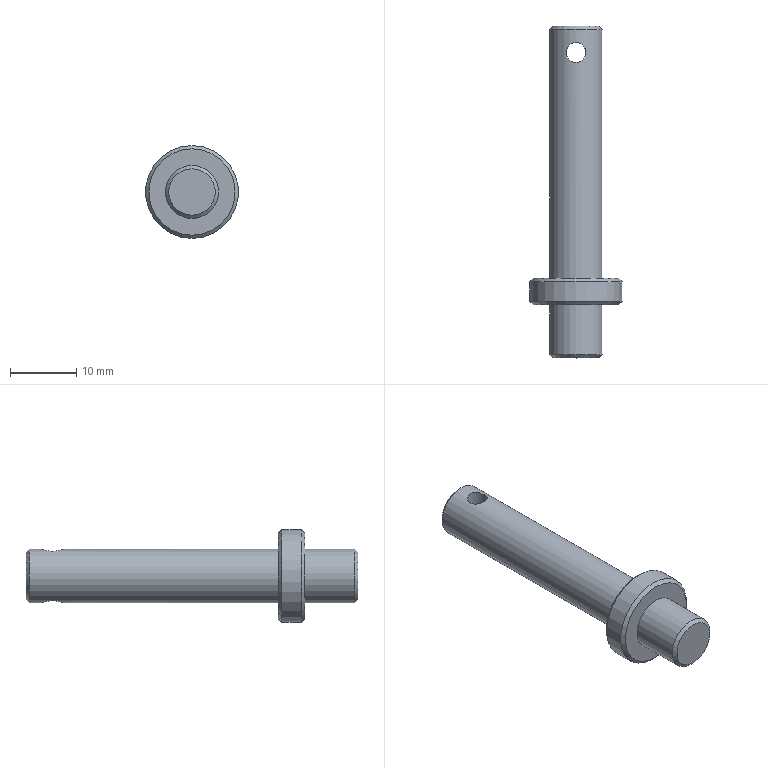Part | NX | features DATUM_CSYS 3, SKETCH 2, CHAMFER 1, EXTRUDE 1, SWP104 1 | 1 solid | 12 faces | box 14 x 50 x 14 mm | volume 2856 mm3 | cylinder 4 | plane 4 | cone 4 | commonest cylinder face diameters 8 x2 3 x1 14 x1
STEP:
#1=CARTESIAN_POINT('',(0.,49.5,-4.));
#2=VERTEX_POINT('',#1);
#3=CARTESIAN_POINT('',(0.,49.5,0.));
#4=DIRECTION('',(0.,-1.,0.));
#5=DIRECTION('',(0.,0.,-1.));
#6=AXIS2_PLACEMENT_3D('',#3,#4,#5);
#7=CIRCLE('',#6,4.);
#8=EDGE_CURVE('',#2,#2,#7,.T.);
#9=ORIENTED_EDGE('',*,*,#8,.T.);
#10=EDGE_LOOP('',(#9));
#11=FACE_BOUND('',#10,.T.);
#12=CARTESIAN_POINT('',(0.,12.,-4.));
#13=VERTEX_POINT('',#12);
#14=CARTESIAN_POINT('',(0.,12.,0.));
#15=DIRECTION('',(0.,-1.,0.));
#16=DIRECTION('',(0.,0.,-1.));
#17=AXIS2_PLACEMENT_3D('',#14,#15,#16);
#18=CIRCLE('',#17,4.);
#19=EDGE_CURVE('',#13,#13,#18,.T.);
#20=ORIENTED_EDGE('',*,*,#19,.F.);
#21=EDGE_LOOP('',(#20));
#22=FACE_BOUND('',#21,.T.);
#23=CARTESIAN_POINT('',(-1.5,46.,3.708));
#24=VERTEX_POINT('',#23);
#25=CARTESIAN_POINT('',(-1.176,47.174,3.859));
#26=CARTESIAN_POINT('',(-1.662,46.,3.632));
#27=CARTESIAN_POINT('',(-1.175,44.825,3.86));
#28=CARTESIAN_POINT('',(-0.002019,44.337,4.07));
#29=CARTESIAN_POINT('',(1.177,44.826,3.859));
#30=CARTESIAN_POINT('',(1.662,45.999,3.632));
#31=CARTESIAN_POINT('',(1.176,47.176,3.86));
#32=CARTESIAN_POINT('',(-0.0004731,47.663,4.07));
#33=CARTESIAN_POINT('',(-1.176,47.174,3.859));
#34=CARTESIAN_POINT('',(-1.662,46.,3.632));
#35=CARTESIAN_POINT('',(-1.175,44.825,3.86));
#36=B_SPLINE_CURVE_WITH_KNOTS('',3,(#25,#26,#27,#28,#29,#30,#31,#32,#33,#34,#35),.UNSPECIFIED.,.T.,.F.,(1,1,1,1,1,1,1,1,1,1,1,1,1,1,1),(-0.003549,-0.002366,-0.001183,0.,0.001183,0.002366,0.003549,0.004733,0.005916,0.007099,0.008282,0.009465,0.01065,0.01183,0.01301),.UNSPECIFIED.);
#37=EDGE_CURVE('',#24,#24,#36,.T.);
#38=ORIENTED_EDGE('',*,*,#37,.F.);
#39=EDGE_LOOP('',(#38));
#40=FACE_BOUND('',#39,.T.);
#41=CARTESIAN_POINT('',(0.,47.5,-4.));
#42=VERTEX_POINT('',#41);
#43=CARTESIAN_POINT('',(-1.175,47.176,-3.86));
#44=CARTESIAN_POINT('',(-0.0003058,47.663,-4.07));
#45=CARTESIAN_POINT('',(1.176,47.174,-3.859));
#46=CARTESIAN_POINT('',(1.662,46.002,-3.632));
#47=CARTESIAN_POINT('',(1.175,44.824,-3.86));
#48=CARTESIAN_POINT('',(0.001125,44.338,-4.07));
#49=CARTESIAN_POINT('',(-1.176,44.825,-3.859));
#50=CARTESIAN_POINT('',(-1.662,46.,-3.632));
#51=CARTESIAN_POINT('',(-1.175,47.176,-3.86));
#52=CARTESIAN_POINT('',(-0.0003058,47.663,-4.07));
#53=CARTESIAN_POINT('',(1.176,47.174,-3.859));
#54=B_SPLINE_CURVE_WITH_KNOTS('',3,(#43,#44,#45,#46,#47,#48,#49,#50,#51,#52,#53),.UNSPECIFIED.,.T.,.F.,(1,1,1,1,1,1,1,1,1,1,1,1,1,1,1),(-0.00355,-0.002366,-0.001183,0.,0.001183,0.002366,0.00355,0.004733,0.005916,0.007099,0.008283,0.009466,0.01065,0.01183,0.01302),.UNSPECIFIED.);
#55=EDGE_CURVE('',#42,#42,#54,.T.);
#56=ORIENTED_EDGE('',*,*,#55,.F.);
#57=EDGE_LOOP('',(#56));
#58=FACE_BOUND('',#57,.T.);
#59=CARTESIAN_POINT('',(0.,50.,0.));
#60=DIRECTION('',(0.,-1.,0.));
#61=DIRECTION('',(0.,0.,-1.));
#62=AXIS2_PLACEMENT_3D('',#59,#60,#61);
#63=CYLINDRICAL_SURFACE('',#62,4.);
#64=ADVANCED_FACE('',(#11,#22,#40,#58),#63,.T.);
#65=CARTESIAN_POINT('',(0.,0.,3.5));
#66=VERTEX_POINT('',#65);
#67=CARTESIAN_POINT('',(0.,0.,0.));
#68=DIRECTION('',(0.,1.,0.));
#69=DIRECTION('',(0.,0.,1.));
#70=AXIS2_PLACEMENT_3D('',#67,#68,#69);
#71=CIRCLE('',#70,3.5);
#72=EDGE_CURVE('',#66,#66,#71,.F.);
#73=ORIENTED_EDGE('',*,*,#72,.T.);
#74=EDGE_LOOP('',(#73));
#75=FACE_BOUND('',#74,.T.);
#76=CARTESIAN_POINT('',(0.,0.,4.));
#77=DIRECTION('',(0.,1.,0.));
#78=DIRECTION('',(0.,0.,1.));
#79=AXIS2_PLACEMENT_3D('',#76,#77,#78);
#80=PLANE('',#79);
#81=ADVANCED_FACE('',(#75),#80,.F.);
#82=CARTESIAN_POINT('',(0.,50.,-3.5));
#83=VERTEX_POINT('',#82);
#84=CARTESIAN_POINT('',(0.,50.,0.));
#85=DIRECTION('',(0.,-1.,0.));
#86=DIRECTION('',(0.,0.,-1.));
#87=AXIS2_PLACEMENT_3D('',#84,#85,#86);
#88=CIRCLE('',#87,3.5);
#89=EDGE_CURVE('',#83,#83,#88,.F.);
#90=ORIENTED_EDGE('',*,*,#89,.T.);
#91=EDGE_LOOP('',(#90));
#92=FACE_BOUND('',#91,.T.);
#93=CARTESIAN_POINT('',(0.,50.,0.));
#94=DIRECTION('',(0.,-1.,0.));
#95=DIRECTION('',(0.,0.,-1.));
#96=AXIS2_PLACEMENT_3D('',#93,#94,#95);
#97=PLANE('',#96);
#98=ADVANCED_FACE('',(#92),#97,.F.);
#99=CARTESIAN_POINT('',(0.,12.,-6.5));
#100=VERTEX_POINT('',#99);
#101=CARTESIAN_POINT('',(0.,12.,0.));
#102=DIRECTION('',(0.,-1.,0.));
#103=DIRECTION('',(0.,0.,-1.));
#104=AXIS2_PLACEMENT_3D('',#101,#102,#103);
#105=CIRCLE('',#104,6.5);
#106=EDGE_CURVE('',#100,#100,#105,.F.);
#107=ORIENTED_EDGE('',*,*,#106,.T.);
#108=EDGE_LOOP('',(#107));
#109=FACE_BOUND('',#108,.T.);
#110=ORIENTED_EDGE('',*,*,#19,.T.);
#111=EDGE_LOOP('',(#110));
#112=FACE_BOUND('',#111,.T.);
#113=CARTESIAN_POINT('',(0.,12.,4.));
#114=DIRECTION('',(0.,-1.,0.));
#115=DIRECTION('',(0.,0.,-1.));
#116=AXIS2_PLACEMENT_3D('',#113,#114,#115);
#117=PLANE('',#116);
#118=ADVANCED_FACE('',(#109,#112),#117,.F.);
#119=CARTESIAN_POINT('',(0.,11.5,-7.));
#120=VERTEX_POINT('',#119);
#121=CARTESIAN_POINT('',(0.,11.5,0.));
#122=DIRECTION('',(0.,-1.,0.));
#123=DIRECTION('',(0.,0.,-1.));
#124=AXIS2_PLACEMENT_3D('',#121,#122,#123);
#125=CIRCLE('',#124,7.);
#126=EDGE_CURVE('',#120,#120,#125,.T.);
#127=ORIENTED_EDGE('',*,*,#126,.T.);
#128=EDGE_LOOP('',(#127));
#129=FACE_BOUND('',#128,.T.);
#130=CARTESIAN_POINT('',(0.,8.5,7.));
#131=VERTEX_POINT('',#130);
#132=CARTESIAN_POINT('',(0.,8.5,0.));
#133=DIRECTION('',(0.,1.,0.));
#134=DIRECTION('',(0.,0.,1.));
#135=AXIS2_PLACEMENT_3D('',#132,#133,#134);
#136=CIRCLE('',#135,7.);
#137=EDGE_CURVE('',#131,#131,#136,.T.);
#138=ORIENTED_EDGE('',*,*,#137,.T.);
#139=EDGE_LOOP('',(#138));
#140=FACE_BOUND('',#139,.T.);
#141=CARTESIAN_POINT('',(0.,50.,0.));
#142=DIRECTION('',(0.,-1.,0.));
#143=DIRECTION('',(0.,0.,-1.));
#144=AXIS2_PLACEMENT_3D('',#141,#142,#143);
#145=CYLINDRICAL_SURFACE('',#144,7.);
#146=ADVANCED_FACE('',(#129,#140),#145,.T.);
#147=CARTESIAN_POINT('',(0.,8.,6.5));
#148=VERTEX_POINT('',#147);
#149=CARTESIAN_POINT('',(0.,8.,0.));
#150=DIRECTION('',(0.,1.,0.));
#151=DIRECTION('',(0.,0.,1.));
#152=AXIS2_PLACEMENT_3D('',#149,#150,#151);
#153=CIRCLE('',#152,6.5);
#154=EDGE_CURVE('',#148,#148,#153,.F.);
#155=ORIENTED_EDGE('',*,*,#154,.T.);
#156=EDGE_LOOP('',(#155));
#157=FACE_BOUND('',#156,.T.);
#158=CARTESIAN_POINT('',(0.,8.,-4.));
#159=VERTEX_POINT('',#158);
#160=CARTESIAN_POINT('',(0.,8.,0.));
#161=DIRECTION('',(0.,-1.,0.));
#162=DIRECTION('',(0.,0.,-1.));
#163=AXIS2_PLACEMENT_3D('',#160,#161,#162);
#164=CIRCLE('',#163,4.);
#165=EDGE_CURVE('',#159,#159,#164,.T.);
#166=ORIENTED_EDGE('',*,*,#165,.F.);
#167=EDGE_LOOP('',(#166));
#168=FACE_BOUND('',#167,.T.);
#169=CARTESIAN_POINT('',(0.,8.,7.));
#170=DIRECTION('',(0.,1.,0.));
#171=DIRECTION('',(0.,0.,1.));
#172=AXIS2_PLACEMENT_3D('',#169,#170,#171);
#173=PLANE('',#172);
#174=ADVANCED_FACE('',(#157,#168),#173,.F.);
#175=CARTESIAN_POINT('',(0.,0.5,4.));
#176=VERTEX_POINT('',#175);
#177=CARTESIAN_POINT('',(0.,0.5,0.));
#178=DIRECTION('',(0.,1.,0.));
#179=DIRECTION('',(0.,0.,1.));
#180=AXIS2_PLACEMENT_3D('',#177,#178,#179);
#181=CIRCLE('',#180,4.);
#182=EDGE_CURVE('',#176,#176,#181,.T.);
#183=ORIENTED_EDGE('',*,*,#182,.T.);
#184=EDGE_LOOP('',(#183));
#185=FACE_BOUND('',#184,.T.);
#186=ORIENTED_EDGE('',*,*,#165,.T.);
#187=EDGE_LOOP('',(#186));
#188=FACE_BOUND('',#187,.T.);
#189=CARTESIAN_POINT('',(0.,50.,0.));
#190=DIRECTION('',(0.,-1.,0.));
#191=DIRECTION('',(0.,0.,-1.));
#192=AXIS2_PLACEMENT_3D('',#189,#190,#191);
#193=CYLINDRICAL_SURFACE('',#192,4.);
#194=ADVANCED_FACE('',(#185,#188),#193,.T.);
#195=ORIENTED_EDGE('',*,*,#37,.T.);
#196=EDGE_LOOP('',(#195));
#197=FACE_BOUND('',#196,.T.);
#198=ORIENTED_EDGE('',*,*,#55,.T.);
#199=EDGE_LOOP('',(#198));
#200=FACE_BOUND('',#199,.T.);
#201=CARTESIAN_POINT('',(0.,46.,8.5));
#202=DIRECTION('',(0.,0.,-1.));
#203=DIRECTION('',(-1.,0.,0.));
#204=AXIS2_PLACEMENT_3D('',#201,#202,#203);
#205=CYLINDRICAL_SURFACE('',#204,1.5);
#206=ADVANCED_FACE('',(#197,#200),#205,.F.);
#207=ORIENTED_EDGE('',*,*,#89,.F.);
#208=EDGE_LOOP('',(#207));
#209=FACE_BOUND('',#208,.T.);
#210=ORIENTED_EDGE('',*,*,#8,.F.);
#211=EDGE_LOOP('',(#210));
#212=FACE_BOUND('',#211,.T.);
#213=CARTESIAN_POINT('',(0.,49.5,0.));
#214=DIRECTION('',(0.,-1.,0.));
#215=DIRECTION('',(0.,0.,-1.));
#216=AXIS2_PLACEMENT_3D('',#213,#214,#215);
#217=CONICAL_SURFACE('',#216,4.,0.7854);
#218=ADVANCED_FACE('',(#209,#212),#217,.T.);
#219=ORIENTED_EDGE('',*,*,#106,.F.);
#220=EDGE_LOOP('',(#219));
#221=FACE_BOUND('',#220,.T.);
#222=ORIENTED_EDGE('',*,*,#126,.F.);
#223=EDGE_LOOP('',(#222));
#224=FACE_BOUND('',#223,.T.);
#225=CARTESIAN_POINT('',(0.,11.5,0.));
#226=DIRECTION('',(0.,-1.,0.));
#227=DIRECTION('',(0.,0.,-1.));
#228=AXIS2_PLACEMENT_3D('',#225,#226,#227);
#229=CONICAL_SURFACE('',#228,7.,0.7854);
#230=ADVANCED_FACE('',(#221,#224),#229,.T.);
#231=ORIENTED_EDGE('',*,*,#137,.F.);
#232=EDGE_LOOP('',(#231));
#233=FACE_BOUND('',#232,.T.);
#234=ORIENTED_EDGE('',*,*,#154,.F.);
#235=EDGE_LOOP('',(#234));
#236=FACE_BOUND('',#235,.T.);
#237=CARTESIAN_POINT('',(0.,8.,0.));
#238=DIRECTION('',(0.,1.,0.));
#239=DIRECTION('',(0.,0.,1.));
#240=AXIS2_PLACEMENT_3D('',#237,#238,#239);
#241=CONICAL_SURFACE('',#240,6.5,0.7854);
#242=ADVANCED_FACE('',(#233,#236),#241,.T.);
#243=ORIENTED_EDGE('',*,*,#182,.F.);
#244=EDGE_LOOP('',(#243));
#245=FACE_BOUND('',#244,.T.);
#246=ORIENTED_EDGE('',*,*,#72,.F.);
#247=EDGE_LOOP('',(#246));
#248=FACE_BOUND('',#247,.T.);
#249=CARTESIAN_POINT('',(0.,0.,0.));
#250=DIRECTION('',(0.,1.,0.));
#251=DIRECTION('',(0.,0.,1.));
#252=AXIS2_PLACEMENT_3D('',#249,#250,#251);
#253=CONICAL_SURFACE('',#252,3.5,0.7854);
#254=ADVANCED_FACE('',(#245,#248),#253,.T.);
#255=CLOSED_SHELL('',(#64,#81,#98,#118,#146,#174,#194,#206,#218,#230,#242,#254));
#256=MANIFOLD_SOLID_BREP('',#255);
#257=(LENGTH_UNIT()NAMED_UNIT(*)SI_UNIT(.MILLI.,.METRE.));
#258=UNCERTAINTY_MEASURE_WITH_UNIT(LENGTH_MEASURE(0.0508),#257,'','');
#259=(NAMED_UNIT(*)PLANE_ANGLE_UNIT()SI_UNIT($,.RADIAN.));
#260=(NAMED_UNIT(*)SI_UNIT($,.STERADIAN.)SOLID_ANGLE_UNIT());
#261=(GEOMETRIC_REPRESENTATION_CONTEXT(3)GLOBAL_UNCERTAINTY_ASSIGNED_CONTEXT((#258))GLOBAL_UNIT_ASSIGNED_CONTEXT((#257,#259,#260))REPRESENTATION_CONTEXT('',''));
#262=ADVANCED_BREP_SHAPE_REPRESENTATION('',(#256),#261);